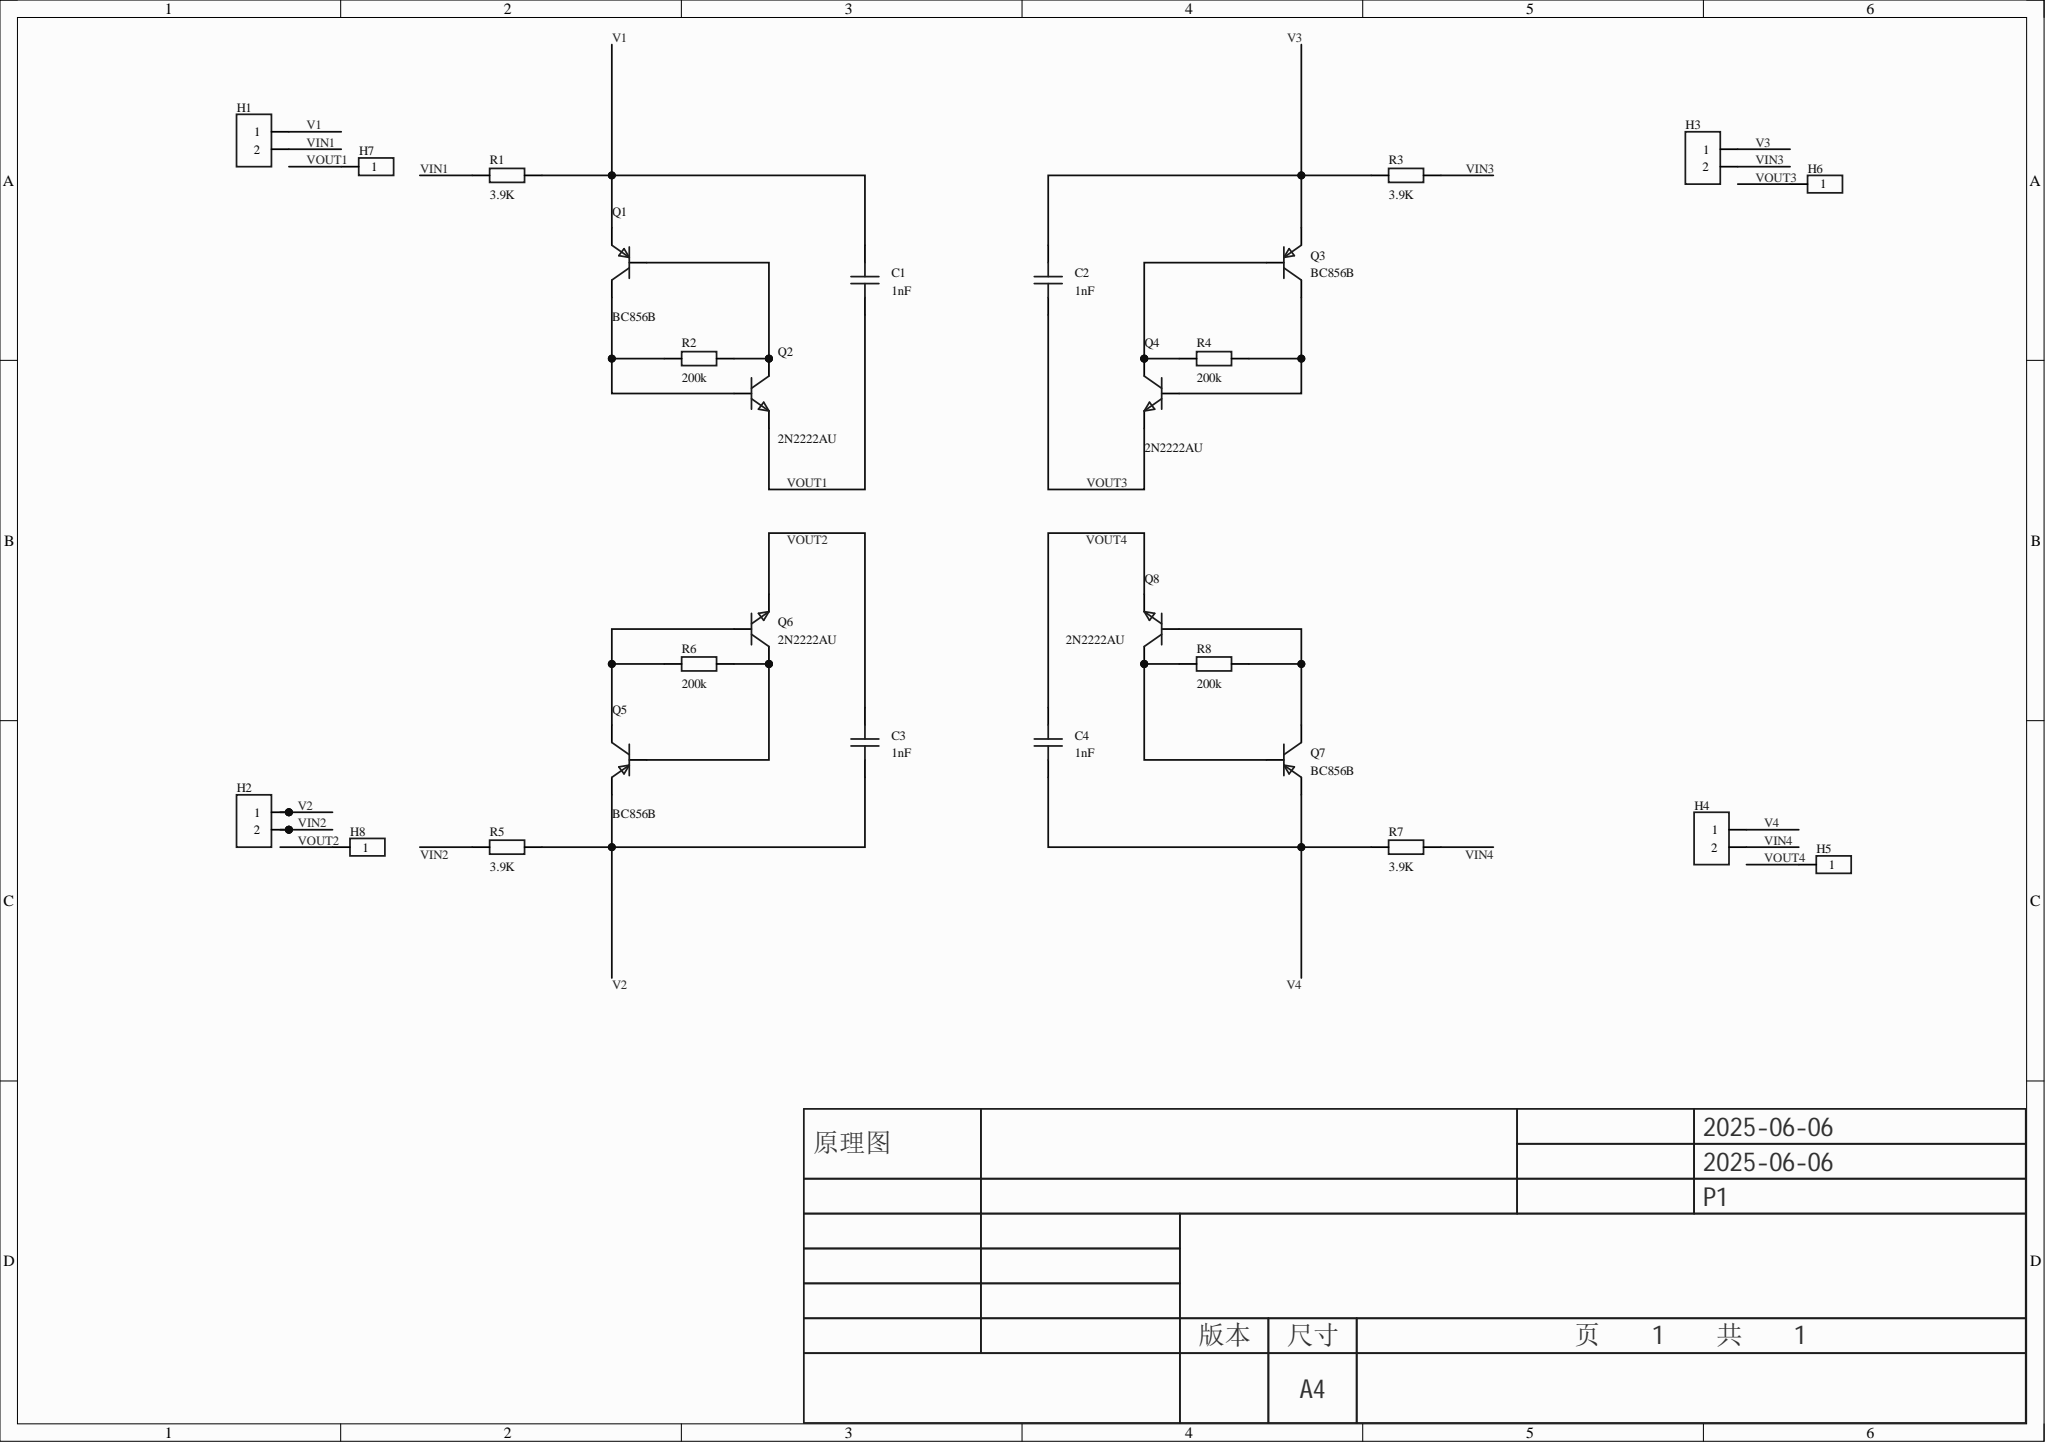Circuit board | Altium Designer | 28 parts | 20 nets
Bill of materials:
Comment,Description,Designator,Footprint,LibRef,Quantity
"1nF","","C1, C2, C3, C4","C0402","CAP_0402","4"
"","","H1, H2, H3, H4","HDR-TH_2P-P2.54-V-F","HDR-F_2.54_1x2P","4"
"","","H5, H6, H7, H8","HDR-TH_1P-V-M_XKB_X4611WV-01I-C28D40","HDR-M_2.54_1x1P","4"
"BC856B","晶体管类型:PNP;集电极电流(Ic):100mA;集射极击穿电压(Vceo):65V;耗散功率(Pd):200mW;直流电流增益(hFE):220@2mA,5V;","Q1, Q3, Q5, Q7","SOT-23-3_L2.9-W1.6-P1.90-LS2.8-BR","BC856B_C181144","4"
"2N2222AU","","Q2, Q4, Q6, Q8","SOT-89-3_L4.5-W2.4-P1.50-LS4.0-BR","2N2222AU","4"
"3.9K","","R1, R3, R5, R7","R0402","Res_0402","4"
"200k","","R2, R4, R6, R8","R0402","Res_0402","4"
Netlist (Protel format):
[
C1
C0402
1nF



]
[
C2
C0402
1nF



]
[
C3
C0402
1nF



]
[
C4
C0402
1nF



]
[
H1
HDR-TH_2P-P2.54-V-F




]
[
H2
HDR-TH_2P-P2.54-V-F




]
[
H3
HDR-TH_2P-P2.54-V-F




]
[
H4
HDR-TH_2P-P2.54-V-F




]
[
H5
HDR-TH_1P-V-M_XKB_X4611WV-01I-C28D40




]
[
H6
HDR-TH_1P-V-M_XKB_X4611WV-01I-C28D40




]
[
H7
HDR-TH_1P-V-M_XKB_X4611WV-01I-C28D40




]
[
H8
HDR-TH_1P-V-M_XKB_X4611WV-01I-C28D40




]
[
Q1
SOT-23-3_L2.9-W1.6-P1.90-LS2.8-BR
BC856B



]
[
Q2
SOT-89-3_L4.5-W2.4-P1.50-LS4.0-BR
2N2222AU



]
[
Q3
SOT-23-3_L2.9-W1.6-P1.90-LS2.8-BR
BC856B



]
[
Q4
SOT-89-3_L4.5-W2.4-P1.50-LS4.0-BR
2N2222AU



]
[
Q5
SOT-23-3_L2.9-W1.6-P1.90-LS2.8-BR
BC856B



]
[
Q6
SOT-89-3_L4.5-W2.4-P1.50-LS4.0-BR
2N2222AU



]
[
Q7
SOT-23-3_L2.9-W1.6-P1.90-LS2.8-BR
BC856B



]
[
Q8
SOT-89-3_L4.5-W2.4-P1.50-LS4.0-BR
2N2222AU



]
[
R1
R0402
3.9K



]
[
R2
R0402
200k



]
[
R3
R0402
3.9K



]
[
R4
R0402
200k



]
[
R5
R0402
3.9K



]
[
R6
R0402
200k



]
[
R7
R0402
3.9K



]
[
R8
R0402
200k



]
(
VOUT4
C4-1
H5-1
Q8-2
)
(
VOUT3
C2-1
H6-1
Q4-2
)
(
VOUT2
C3-1
H8-1
Q6-2
)
(
VOUT1
C1-1
H7-1
Q2-2
)
(
VIN4
H4-2
R7-1
)
(
VIN3
H3-2
R3-1
)
(
VIN2
H2-2
R5-1
)
(
VIN1
H1-2
R1-1
)
(
V4
C4-2
H4-1
Q7-2
R7-2
)
(
V3
C2-2
H3-1
Q3-2
R3-2
)
(
V2
C3-2
H2-1
Q5-2
R5-2
)
(
V1
C1-2
H1-1
Q1-2
R1-2
)
(
NetQ7_3
Q7-3
Q8-1
R8-1
)
(
NetQ7_1
Q7-1
Q8-3
R8-2
)
(
NetQ5_3
Q5-3
Q6-1
R6-1
)
(
NetQ5_1
Q5-1
Q6-3
R6-2
)
(
NetQ3_3
Q3-3
Q4-1
R4-1
)
(
NetQ3_1
Q3-1
Q4-3
R4-2
)
(
NetQ1_3
Q1-3
Q2-1
R2-1
)
(
NetQ1_1
Q1-1
Q2-3
R2-2
)